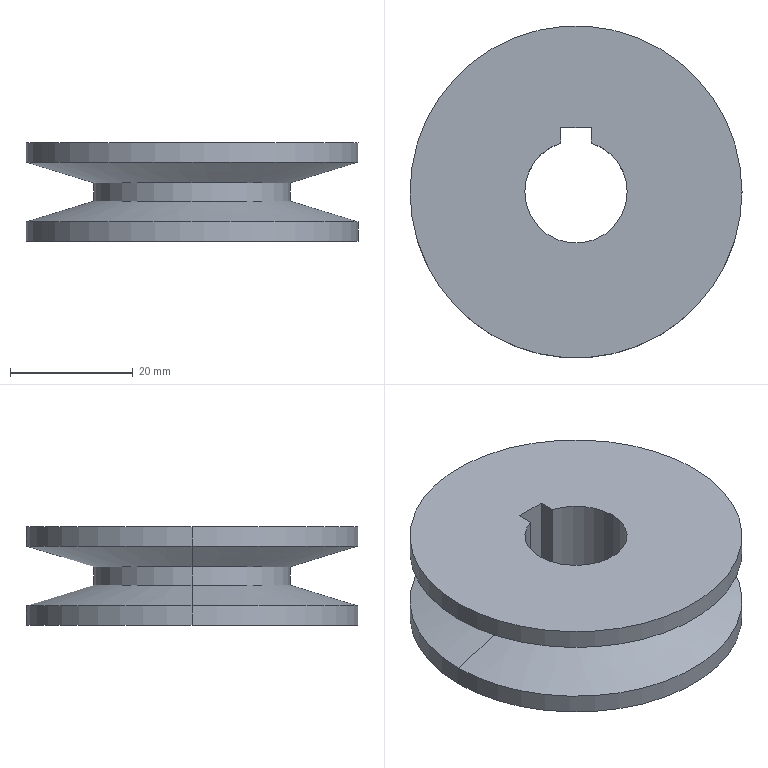Part | SolidWorks | features ICE 2, BaseBody 1 | 1 solid | 18 faces | box 54 x 54 x 16 mm | volume 23103 mm3 | cylinder 9 | plane 5 | cone 4 | commonest cylinder face diameters 54 x4 16.64 x3 32 x2
STEP:
#1=CARTESIAN_POINT('',(-8.32,0.,0.));
#2=VERTEX_POINT('',#1);
#3=CARTESIAN_POINT('',(8.32,0.,0.));
#4=VERTEX_POINT('',#3);
#5=CARTESIAN_POINT('',(0.,0.,0.));
#6=DIRECTION('',(0.,0.,1.));
#7=DIRECTION('',(1.,0.,0.));
#8=AXIS2_PLACEMENT_3D('',#5,#6,#7);
#9=CIRCLE('',#8,8.32);
#10=EDGE_CURVE('',#2,#4,#9,.T.);
#11=ORIENTED_EDGE('',*,*,#10,.F.);
#12=CARTESIAN_POINT('',(-8.32,0.,16.));
#13=VERTEX_POINT('',#12);
#14=CARTESIAN_POINT('',(-8.32,0.,0.));
#15=DIRECTION('',(0.,0.,1.));
#16=VECTOR('',#15,1000.);
#17=LINE('',#14,#16);
#18=EDGE_CURVE('',#2,#13,#17,.T.);
#19=ORIENTED_EDGE('',*,*,#18,.T.);
#20=CARTESIAN_POINT('',(8.32,0.,16.));
#21=VERTEX_POINT('',#20);
#22=CARTESIAN_POINT('',(0.,0.,16.));
#23=DIRECTION('',(0.,0.,1.));
#24=DIRECTION('',(1.,0.,0.));
#25=AXIS2_PLACEMENT_3D('',#22,#23,#24);
#26=CIRCLE('',#25,8.32);
#27=EDGE_CURVE('',#13,#21,#26,.T.);
#28=ORIENTED_EDGE('',*,*,#27,.T.);
#29=CARTESIAN_POINT('',(8.32,0.,0.));
#30=DIRECTION('',(0.,0.,1.));
#31=VECTOR('',#30,1000.);
#32=LINE('',#29,#31);
#33=EDGE_CURVE('',#4,#21,#32,.T.);
#34=ORIENTED_EDGE('',*,*,#33,.F.);
#35=EDGE_LOOP('',(#11,#19,#28,#34));
#36=FACE_OUTER_BOUND('',#35,.T.);
#37=CARTESIAN_POINT('',(0.,0.,0.));
#38=DIRECTION('',(0.,0.,1.));
#39=DIRECTION('',(1.,0.,0.));
#40=AXIS2_PLACEMENT_3D('',#37,#38,#39);
#41=CYLINDRICAL_SURFACE('',#40,8.32);
#42=ADVANCED_FACE('',(#36),#41,.F.);
#43=CARTESIAN_POINT('',(2.5,7.936,0.));
#44=VERTEX_POINT('',#43);
#45=CARTESIAN_POINT('',(0.,0.,0.));
#46=DIRECTION('',(0.,0.,1.));
#47=DIRECTION('',(1.,0.,0.));
#48=AXIS2_PLACEMENT_3D('',#45,#46,#47);
#49=CIRCLE('',#48,8.32);
#50=EDGE_CURVE('',#4,#44,#49,.T.);
#51=ORIENTED_EDGE('',*,*,#50,.F.);
#52=ORIENTED_EDGE('',*,*,#33,.T.);
#53=CARTESIAN_POINT('',(2.5,7.936,16.));
#54=VERTEX_POINT('',#53);
#55=CARTESIAN_POINT('',(0.,0.,16.));
#56=DIRECTION('',(0.,0.,1.));
#57=DIRECTION('',(1.,0.,0.));
#58=AXIS2_PLACEMENT_3D('',#55,#56,#57);
#59=CIRCLE('',#58,8.32);
#60=EDGE_CURVE('',#21,#54,#59,.T.);
#61=ORIENTED_EDGE('',*,*,#60,.T.);
#62=CARTESIAN_POINT('',(2.5,7.936,0.));
#63=DIRECTION('',(0.,0.,-1.));
#64=VECTOR('',#63,1000.);
#65=LINE('',#62,#64);
#66=EDGE_CURVE('',#54,#44,#65,.T.);
#67=ORIENTED_EDGE('',*,*,#66,.T.);
#68=EDGE_LOOP('',(#51,#52,#61,#67));
#69=FACE_OUTER_BOUND('',#68,.T.);
#70=CARTESIAN_POINT('',(0.,0.,0.));
#71=DIRECTION('',(0.,0.,1.));
#72=DIRECTION('',(1.,0.,0.));
#73=AXIS2_PLACEMENT_3D('',#70,#71,#72);
#74=CYLINDRICAL_SURFACE('',#73,8.32);
#75=ADVANCED_FACE('',(#69),#74,.F.);
#76=CARTESIAN_POINT('',(27.,0.,16.));
#77=VERTEX_POINT('',#76);
#78=CARTESIAN_POINT('',(-27.,0.,16.));
#79=VERTEX_POINT('',#78);
#80=CARTESIAN_POINT('',(0.,0.,16.));
#81=DIRECTION('',(0.,0.,1.));
#82=DIRECTION('',(-1.,0.,0.));
#83=AXIS2_PLACEMENT_3D('',#80,#81,#82);
#84=CIRCLE('',#83,27.);
#85=EDGE_CURVE('',#77,#79,#84,.T.);
#86=ORIENTED_EDGE('',*,*,#85,.F.);
#87=CARTESIAN_POINT('',(27.,0.,12.861));
#88=VERTEX_POINT('',#87);
#89=CARTESIAN_POINT('',(27.,0.,8.));
#90=DIRECTION('',(0.,0.,-1.));
#91=VECTOR('',#90,1000.);
#92=LINE('',#89,#91);
#93=EDGE_CURVE('',#77,#88,#92,.T.);
#94=ORIENTED_EDGE('',*,*,#93,.T.);
#95=CARTESIAN_POINT('',(-27.,0.,12.861));
#96=VERTEX_POINT('',#95);
#97=CARTESIAN_POINT('',(0.,0.,12.861));
#98=DIRECTION('',(0.,0.,1.));
#99=DIRECTION('',(-1.,0.,0.));
#100=AXIS2_PLACEMENT_3D('',#97,#98,#99);
#101=CIRCLE('',#100,27.);
#102=EDGE_CURVE('',#88,#96,#101,.T.);
#103=ORIENTED_EDGE('',*,*,#102,.T.);
#104=CARTESIAN_POINT('',(-27.,0.,8.));
#105=DIRECTION('',(0.,0.,-1.));
#106=VECTOR('',#105,1000.);
#107=LINE('',#104,#106);
#108=EDGE_CURVE('',#79,#96,#107,.T.);
#109=ORIENTED_EDGE('',*,*,#108,.F.);
#110=EDGE_LOOP('',(#86,#94,#103,#109));
#111=FACE_OUTER_BOUND('',#110,.T.);
#112=CARTESIAN_POINT('',(0.,0.,8.));
#113=DIRECTION('',(0.,0.,-1.));
#114=DIRECTION('',(-1.,0.,0.));
#115=AXIS2_PLACEMENT_3D('',#112,#113,#114);
#116=CYLINDRICAL_SURFACE('',#115,27.);
#117=ADVANCED_FACE('',(#111),#116,.T.);
#118=CARTESIAN_POINT('',(16.,0.,9.498));
#119=VERTEX_POINT('',#118);
#120=CARTESIAN_POINT('',(-16.,0.,9.498));
#121=VERTEX_POINT('',#120);
#122=CARTESIAN_POINT('',(0.,0.,9.498));
#123=DIRECTION('',(0.,0.,1.));
#124=DIRECTION('',(0.,1.,0.));
#125=AXIS2_PLACEMENT_3D('',#122,#123,#124);
#126=CIRCLE('',#125,16.);
#127=EDGE_CURVE('',#119,#121,#126,.T.);
#128=ORIENTED_EDGE('',*,*,#127,.T.);
#129=CARTESIAN_POINT('',(-27.,0.,12.861));
#130=DIRECTION('',(-0.9563,0.,0.2924));
#131=VECTOR('',#130,1000.);
#132=LINE('',#129,#131);
#133=EDGE_CURVE('',#121,#96,#132,.T.);
#134=ORIENTED_EDGE('',*,*,#133,.T.);
#135=ORIENTED_EDGE('',*,*,#102,.F.);
#136=CARTESIAN_POINT('',(27.,0.,12.861));
#137=DIRECTION('',(0.9563,0.,0.2924));
#138=VECTOR('',#137,1000.);
#139=LINE('',#136,#138);
#140=EDGE_CURVE('',#119,#88,#139,.T.);
#141=ORIENTED_EDGE('',*,*,#140,.F.);
#142=EDGE_LOOP('',(#128,#134,#135,#141));
#143=FACE_OUTER_BOUND('',#142,.T.);
#144=CARTESIAN_POINT('',(0.,0.,12.861));
#145=DIRECTION('',(0.,0.,1.));
#146=DIRECTION('',(1.,0.,0.));
#147=AXIS2_PLACEMENT_3D('',#144,#145,#146);
#148=CONICAL_SURFACE('',#147,27.,1.274);
#149=ADVANCED_FACE('',(#143),#148,.T.);
#150=CARTESIAN_POINT('',(16.,0.,6.502));
#151=VERTEX_POINT('',#150);
#152=CARTESIAN_POINT('',(-16.,0.,6.502));
#153=VERTEX_POINT('',#152);
#154=CARTESIAN_POINT('',(0.,0.,6.502));
#155=DIRECTION('',(0.,0.,1.));
#156=DIRECTION('',(1.,0.,0.));
#157=AXIS2_PLACEMENT_3D('',#154,#155,#156);
#158=CIRCLE('',#157,16.);
#159=EDGE_CURVE('',#151,#153,#158,.T.);
#160=ORIENTED_EDGE('',*,*,#159,.T.);
#161=CARTESIAN_POINT('',(-16.,0.,8.));
#162=DIRECTION('',(0.,0.,1.));
#163=VECTOR('',#162,1000.);
#164=LINE('',#161,#163);
#165=EDGE_CURVE('',#153,#121,#164,.T.);
#166=ORIENTED_EDGE('',*,*,#165,.T.);
#167=ORIENTED_EDGE('',*,*,#127,.F.);
#168=CARTESIAN_POINT('',(16.,0.,8.));
#169=DIRECTION('',(0.,0.,1.));
#170=VECTOR('',#169,1000.);
#171=LINE('',#168,#170);
#172=EDGE_CURVE('',#151,#119,#171,.T.);
#173=ORIENTED_EDGE('',*,*,#172,.F.);
#174=EDGE_LOOP('',(#160,#166,#167,#173));
#175=FACE_OUTER_BOUND('',#174,.T.);
#176=CARTESIAN_POINT('',(0.,0.,8.));
#177=DIRECTION('',(0.,0.,1.));
#178=DIRECTION('',(1.,0.,0.));
#179=AXIS2_PLACEMENT_3D('',#176,#177,#178);
#180=CYLINDRICAL_SURFACE('',#179,16.);
#181=ADVANCED_FACE('',(#175),#180,.T.);
#182=ORIENTED_EDGE('',*,*,#159,.F.);
#183=CARTESIAN_POINT('',(27.,0.,3.139));
#184=VERTEX_POINT('',#183);
#185=CARTESIAN_POINT('',(27.,0.,3.139));
#186=DIRECTION('',(0.9563,0.,-0.2924));
#187=VECTOR('',#186,1000.);
#188=LINE('',#185,#187);
#189=EDGE_CURVE('',#151,#184,#188,.T.);
#190=ORIENTED_EDGE('',*,*,#189,.T.);
#191=CARTESIAN_POINT('',(-27.,0.,3.139));
#192=VERTEX_POINT('',#191);
#193=CARTESIAN_POINT('',(0.,0.,3.139));
#194=DIRECTION('',(0.,0.,1.));
#195=DIRECTION('',(0.,1.,0.));
#196=AXIS2_PLACEMENT_3D('',#193,#194,#195);
#197=CIRCLE('',#196,27.);
#198=EDGE_CURVE('',#184,#192,#197,.T.);
#199=ORIENTED_EDGE('',*,*,#198,.T.);
#200=CARTESIAN_POINT('',(-27.,0.,3.139));
#201=DIRECTION('',(-0.9563,0.,-0.2924));
#202=VECTOR('',#201,1000.);
#203=LINE('',#200,#202);
#204=EDGE_CURVE('',#153,#192,#203,.T.);
#205=ORIENTED_EDGE('',*,*,#204,.F.);
#206=EDGE_LOOP('',(#182,#190,#199,#205));
#207=FACE_OUTER_BOUND('',#206,.T.);
#208=CARTESIAN_POINT('',(0.,0.,3.139));
#209=DIRECTION('',(0.,0.,-1.));
#210=DIRECTION('',(-1.,0.,0.));
#211=AXIS2_PLACEMENT_3D('',#208,#209,#210);
#212=CONICAL_SURFACE('',#211,27.,1.274);
#213=ADVANCED_FACE('',(#207),#212,.T.);
#214=ORIENTED_EDGE('',*,*,#198,.F.);
#215=CARTESIAN_POINT('',(27.,0.,0.));
#216=VERTEX_POINT('',#215);
#217=CARTESIAN_POINT('',(27.,0.,8.));
#218=DIRECTION('',(0.,0.,-1.));
#219=VECTOR('',#218,1000.);
#220=LINE('',#217,#219);
#221=EDGE_CURVE('',#184,#216,#220,.T.);
#222=ORIENTED_EDGE('',*,*,#221,.T.);
#223=CARTESIAN_POINT('',(-27.,0.,0.));
#224=VERTEX_POINT('',#223);
#225=CARTESIAN_POINT('',(0.,0.,0.));
#226=DIRECTION('',(0.,0.,1.));
#227=DIRECTION('',(-1.,0.,0.));
#228=AXIS2_PLACEMENT_3D('',#225,#226,#227);
#229=CIRCLE('',#228,27.);
#230=EDGE_CURVE('',#216,#224,#229,.T.);
#231=ORIENTED_EDGE('',*,*,#230,.T.);
#232=CARTESIAN_POINT('',(-27.,0.,8.));
#233=DIRECTION('',(0.,0.,-1.));
#234=VECTOR('',#233,1000.);
#235=LINE('',#232,#234);
#236=EDGE_CURVE('',#192,#224,#235,.T.);
#237=ORIENTED_EDGE('',*,*,#236,.F.);
#238=EDGE_LOOP('',(#214,#222,#231,#237));
#239=FACE_OUTER_BOUND('',#238,.T.);
#240=CARTESIAN_POINT('',(0.,0.,8.));
#241=DIRECTION('',(0.,0.,-1.));
#242=DIRECTION('',(-1.,0.,0.));
#243=AXIS2_PLACEMENT_3D('',#240,#241,#242);
#244=CYLINDRICAL_SURFACE('',#243,27.);
#245=ADVANCED_FACE('',(#239),#244,.T.);
#246=CARTESIAN_POINT('',(-2.5,10.5,16.));
#247=VERTEX_POINT('',#246);
#248=CARTESIAN_POINT('',(-2.5,7.936,16.));
#249=VERTEX_POINT('',#248);
#250=CARTESIAN_POINT('',(-2.5,10.5,16.));
#251=DIRECTION('',(0.,-1.,0.));
#252=VECTOR('',#251,1000.);
#253=LINE('',#250,#252);
#254=EDGE_CURVE('',#247,#249,#253,.T.);
#255=ORIENTED_EDGE('',*,*,#254,.F.);
#256=CARTESIAN_POINT('',(2.5,10.5,16.));
#257=VERTEX_POINT('',#256);
#258=CARTESIAN_POINT('',(-2.5,10.5,16.));
#259=DIRECTION('',(-1.,0.,0.));
#260=VECTOR('',#259,1000.);
#261=LINE('',#258,#260);
#262=EDGE_CURVE('',#257,#247,#261,.T.);
#263=ORIENTED_EDGE('',*,*,#262,.F.);
#264=CARTESIAN_POINT('',(2.5,10.5,16.));
#265=DIRECTION('',(0.,1.,0.));
#266=VECTOR('',#265,1000.);
#267=LINE('',#264,#266);
#268=EDGE_CURVE('',#54,#257,#267,.T.);
#269=ORIENTED_EDGE('',*,*,#268,.F.);
#270=ORIENTED_EDGE('',*,*,#60,.F.);
#271=ORIENTED_EDGE('',*,*,#27,.F.);
#272=CARTESIAN_POINT('',(0.,0.,16.));
#273=DIRECTION('',(0.,0.,1.));
#274=DIRECTION('',(1.,0.,0.));
#275=AXIS2_PLACEMENT_3D('',#272,#273,#274);
#276=CIRCLE('',#275,8.32);
#277=EDGE_CURVE('',#249,#13,#276,.T.);
#278=ORIENTED_EDGE('',*,*,#277,.F.);
#279=EDGE_LOOP('',(#255,#263,#269,#270,#271,#278));
#280=FACE_BOUND('',#279,.T.);
#281=CARTESIAN_POINT('',(0.,0.,16.));
#282=DIRECTION('',(0.,0.,1.));
#283=DIRECTION('',(-1.,0.,0.));
#284=AXIS2_PLACEMENT_3D('',#281,#282,#283);
#285=CIRCLE('',#284,27.);
#286=EDGE_CURVE('',#79,#77,#285,.T.);
#287=ORIENTED_EDGE('',*,*,#286,.T.);
#288=ORIENTED_EDGE('',*,*,#85,.T.);
#289=EDGE_LOOP('',(#287,#288));
#290=FACE_OUTER_BOUND('',#289,.T.);
#291=CARTESIAN_POINT('',(0.,13.5,16.));
#292=DIRECTION('',(0.,0.,1.));
#293=DIRECTION('',(1.,0.,0.));
#294=AXIS2_PLACEMENT_3D('',#291,#292,#293);
#295=PLANE('',#294);
#296=ADVANCED_FACE('',(#280,#290),#295,.T.);
#297=ORIENTED_EDGE('',*,*,#93,.F.);
#298=ORIENTED_EDGE('',*,*,#286,.F.);
#299=ORIENTED_EDGE('',*,*,#108,.T.);
#300=CARTESIAN_POINT('',(0.,0.,12.861));
#301=DIRECTION('',(0.,0.,1.));
#302=DIRECTION('',(-1.,0.,0.));
#303=AXIS2_PLACEMENT_3D('',#300,#301,#302);
#304=CIRCLE('',#303,27.);
#305=EDGE_CURVE('',#96,#88,#304,.T.);
#306=ORIENTED_EDGE('',*,*,#305,.T.);
#307=EDGE_LOOP('',(#297,#298,#299,#306));
#308=FACE_OUTER_BOUND('',#307,.T.);
#309=CARTESIAN_POINT('',(0.,0.,8.));
#310=DIRECTION('',(0.,0.,-1.));
#311=DIRECTION('',(-1.,0.,0.));
#312=AXIS2_PLACEMENT_3D('',#309,#310,#311);
#313=CYLINDRICAL_SURFACE('',#312,27.);
#314=ADVANCED_FACE('',(#308),#313,.T.);
#315=ORIENTED_EDGE('',*,*,#133,.F.);
#316=CARTESIAN_POINT('',(0.,0.,9.498));
#317=DIRECTION('',(0.,0.,1.));
#318=DIRECTION('',(0.,1.,0.));
#319=AXIS2_PLACEMENT_3D('',#316,#317,#318);
#320=CIRCLE('',#319,16.);
#321=EDGE_CURVE('',#121,#119,#320,.T.);
#322=ORIENTED_EDGE('',*,*,#321,.T.);
#323=ORIENTED_EDGE('',*,*,#140,.T.);
#324=ORIENTED_EDGE('',*,*,#305,.F.);
#325=EDGE_LOOP('',(#315,#322,#323,#324));
#326=FACE_OUTER_BOUND('',#325,.T.);
#327=CARTESIAN_POINT('',(0.,0.,12.861));
#328=DIRECTION('',(0.,0.,1.));
#329=DIRECTION('',(1.,0.,0.));
#330=AXIS2_PLACEMENT_3D('',#327,#328,#329);
#331=CONICAL_SURFACE('',#330,27.,1.274);
#332=ADVANCED_FACE('',(#326),#331,.T.);
#333=ORIENTED_EDGE('',*,*,#165,.F.);
#334=CARTESIAN_POINT('',(0.,0.,6.502));
#335=DIRECTION('',(0.,0.,1.));
#336=DIRECTION('',(1.,0.,0.));
#337=AXIS2_PLACEMENT_3D('',#334,#335,#336);
#338=CIRCLE('',#337,16.);
#339=EDGE_CURVE('',#153,#151,#338,.T.);
#340=ORIENTED_EDGE('',*,*,#339,.T.);
#341=ORIENTED_EDGE('',*,*,#172,.T.);
#342=ORIENTED_EDGE('',*,*,#321,.F.);
#343=EDGE_LOOP('',(#333,#340,#341,#342));
#344=FACE_OUTER_BOUND('',#343,.T.);
#345=CARTESIAN_POINT('',(0.,0.,8.));
#346=DIRECTION('',(0.,0.,1.));
#347=DIRECTION('',(1.,0.,0.));
#348=AXIS2_PLACEMENT_3D('',#345,#346,#347);
#349=CYLINDRICAL_SURFACE('',#348,16.);
#350=ADVANCED_FACE('',(#344),#349,.T.);
#351=ORIENTED_EDGE('',*,*,#189,.F.);
#352=ORIENTED_EDGE('',*,*,#339,.F.);
#353=ORIENTED_EDGE('',*,*,#204,.T.);
#354=CARTESIAN_POINT('',(0.,0.,3.139));
#355=DIRECTION('',(0.,0.,1.));
#356=DIRECTION('',(0.,1.,0.));
#357=AXIS2_PLACEMENT_3D('',#354,#355,#356);
#358=CIRCLE('',#357,27.);
#359=EDGE_CURVE('',#192,#184,#358,.T.);
#360=ORIENTED_EDGE('',*,*,#359,.T.);
#361=EDGE_LOOP('',(#351,#352,#353,#360));
#362=FACE_OUTER_BOUND('',#361,.T.);
#363=CARTESIAN_POINT('',(0.,0.,3.139));
#364=DIRECTION('',(0.,0.,-1.));
#365=DIRECTION('',(-1.,0.,0.));
#366=AXIS2_PLACEMENT_3D('',#363,#364,#365);
#367=CONICAL_SURFACE('',#366,27.,1.274);
#368=ADVANCED_FACE('',(#362),#367,.T.);
#369=ORIENTED_EDGE('',*,*,#221,.F.);
#370=ORIENTED_EDGE('',*,*,#359,.F.);
#371=ORIENTED_EDGE('',*,*,#236,.T.);
#372=CARTESIAN_POINT('',(0.,0.,0.));
#373=DIRECTION('',(0.,0.,1.));
#374=DIRECTION('',(-1.,0.,0.));
#375=AXIS2_PLACEMENT_3D('',#372,#373,#374);
#376=CIRCLE('',#375,27.);
#377=EDGE_CURVE('',#224,#216,#376,.T.);
#378=ORIENTED_EDGE('',*,*,#377,.T.);
#379=EDGE_LOOP('',(#369,#370,#371,#378));
#380=FACE_OUTER_BOUND('',#379,.T.);
#381=CARTESIAN_POINT('',(0.,0.,8.));
#382=DIRECTION('',(0.,0.,-1.));
#383=DIRECTION('',(-1.,0.,0.));
#384=AXIS2_PLACEMENT_3D('',#381,#382,#383);
#385=CYLINDRICAL_SURFACE('',#384,27.);
#386=ADVANCED_FACE('',(#380),#385,.T.);
#387=CARTESIAN_POINT('',(-2.5,10.5,0.));
#388=VERTEX_POINT('',#387);
#389=CARTESIAN_POINT('',(-2.5,7.936,0.));
#390=VERTEX_POINT('',#389);
#391=CARTESIAN_POINT('',(-2.5,10.5,0.));
#392=DIRECTION('',(0.,-1.,0.));
#393=VECTOR('',#392,1000.);
#394=LINE('',#391,#393);
#395=EDGE_CURVE('',#388,#390,#394,.T.);
#396=ORIENTED_EDGE('',*,*,#395,.T.);
#397=CARTESIAN_POINT('',(0.,0.,0.));
#398=DIRECTION('',(0.,0.,1.));
#399=DIRECTION('',(1.,0.,0.));
#400=AXIS2_PLACEMENT_3D('',#397,#398,#399);
#401=CIRCLE('',#400,8.32);
#402=EDGE_CURVE('',#390,#2,#401,.T.);
#403=ORIENTED_EDGE('',*,*,#402,.T.);
#404=ORIENTED_EDGE('',*,*,#10,.T.);
#405=ORIENTED_EDGE('',*,*,#50,.T.);
#406=CARTESIAN_POINT('',(2.5,10.5,0.));
#407=VERTEX_POINT('',#406);
#408=CARTESIAN_POINT('',(2.5,10.5,0.));
#409=DIRECTION('',(0.,1.,0.));
#410=VECTOR('',#409,1000.);
#411=LINE('',#408,#410);
#412=EDGE_CURVE('',#44,#407,#411,.T.);
#413=ORIENTED_EDGE('',*,*,#412,.T.);
#414=CARTESIAN_POINT('',(-2.5,10.5,0.));
#415=DIRECTION('',(-1.,0.,0.));
#416=VECTOR('',#415,1000.);
#417=LINE('',#414,#416);
#418=EDGE_CURVE('',#407,#388,#417,.T.);
#419=ORIENTED_EDGE('',*,*,#418,.T.);
#420=EDGE_LOOP('',(#396,#403,#404,#405,#413,#419));
#421=FACE_BOUND('',#420,.T.);
#422=ORIENTED_EDGE('',*,*,#377,.F.);
#423=ORIENTED_EDGE('',*,*,#230,.F.);
#424=EDGE_LOOP('',(#422,#423));
#425=FACE_OUTER_BOUND('',#424,.T.);
#426=CARTESIAN_POINT('',(0.,13.5,0.));
#427=DIRECTION('',(0.,0.,-1.));
#428=DIRECTION('',(-1.,0.,0.));
#429=AXIS2_PLACEMENT_3D('',#426,#427,#428);
#430=PLANE('',#429);
#431=ADVANCED_FACE('',(#421,#425),#430,.T.);
#432=ORIENTED_EDGE('',*,*,#18,.F.);
#433=ORIENTED_EDGE('',*,*,#402,.F.);
#434=CARTESIAN_POINT('',(-2.5,7.936,0.));
#435=DIRECTION('',(0.,0.,1.));
#436=VECTOR('',#435,1000.);
#437=LINE('',#434,#436);
#438=EDGE_CURVE('',#390,#249,#437,.T.);
#439=ORIENTED_EDGE('',*,*,#438,.T.);
#440=ORIENTED_EDGE('',*,*,#277,.T.);
#441=EDGE_LOOP('',(#432,#433,#439,#440));
#442=FACE_OUTER_BOUND('',#441,.T.);
#443=CARTESIAN_POINT('',(0.,0.,0.));
#444=DIRECTION('',(0.,0.,1.));
#445=DIRECTION('',(1.,0.,0.));
#446=AXIS2_PLACEMENT_3D('',#443,#444,#445);
#447=CYLINDRICAL_SURFACE('',#446,8.32);
#448=ADVANCED_FACE('',(#442),#447,.F.);
#449=ORIENTED_EDGE('',*,*,#395,.F.);
#450=CARTESIAN_POINT('',(-2.5,10.5,0.));
#451=DIRECTION('',(0.,0.,1.));
#452=VECTOR('',#451,1000.);
#453=LINE('',#450,#452);
#454=EDGE_CURVE('',#388,#247,#453,.T.);
#455=ORIENTED_EDGE('',*,*,#454,.T.);
#456=ORIENTED_EDGE('',*,*,#254,.T.);
#457=ORIENTED_EDGE('',*,*,#438,.F.);
#458=EDGE_LOOP('',(#449,#455,#456,#457));
#459=FACE_OUTER_BOUND('',#458,.T.);
#460=CARTESIAN_POINT('',(-2.5,10.5,0.));
#461=DIRECTION('',(-1.,0.,0.));
#462=DIRECTION('',(0.,-1.,0.));
#463=AXIS2_PLACEMENT_3D('',#460,#461,#462);
#464=PLANE('',#463);
#465=ADVANCED_FACE('',(#459),#464,.F.);
#466=ORIENTED_EDGE('',*,*,#268,.T.);
#467=CARTESIAN_POINT('',(2.5,10.5,0.));
#468=DIRECTION('',(0.,0.,1.));
#469=VECTOR('',#468,1000.);
#470=LINE('',#467,#469);
#471=EDGE_CURVE('',#407,#257,#470,.T.);
#472=ORIENTED_EDGE('',*,*,#471,.F.);
#473=ORIENTED_EDGE('',*,*,#412,.F.);
#474=ORIENTED_EDGE('',*,*,#66,.F.);
#475=EDGE_LOOP('',(#466,#472,#473,#474));
#476=FACE_OUTER_BOUND('',#475,.T.);
#477=CARTESIAN_POINT('',(2.5,10.5,0.));
#478=DIRECTION('',(1.,0.,0.));
#479=DIRECTION('',(0.,1.,0.));
#480=AXIS2_PLACEMENT_3D('',#477,#478,#479);
#481=PLANE('',#480);
#482=ADVANCED_FACE('',(#476),#481,.F.);
#483=ORIENTED_EDGE('',*,*,#262,.T.);
#484=ORIENTED_EDGE('',*,*,#454,.F.);
#485=ORIENTED_EDGE('',*,*,#418,.F.);
#486=ORIENTED_EDGE('',*,*,#471,.T.);
#487=EDGE_LOOP('',(#483,#484,#485,#486));
#488=FACE_OUTER_BOUND('',#487,.T.);
#489=CARTESIAN_POINT('',(-2.5,10.5,0.));
#490=DIRECTION('',(0.,1.,0.));
#491=DIRECTION('',(0.,0.,1.));
#492=AXIS2_PLACEMENT_3D('',#489,#490,#491);
#493=PLANE('',#492);
#494=ADVANCED_FACE('',(#488),#493,.F.);
#495=CLOSED_SHELL('',(#42,#75,#117,#149,#181,#213,#245,#296,#314,#332,#350,#368,#386,#431,#448,#465,#482,#494));
#496=MANIFOLD_SOLID_BREP('',#495);
#497=CARTESIAN_POINT('',(0.,0.,0.));
#498=DIRECTION('',(0.,0.,1.));
#499=DIRECTION('',(1.,0.,0.));
#500=AXIS2_PLACEMENT_3D('',#497,#498,#499);
#501=(LENGTH_UNIT()NAMED_UNIT(*)SI_UNIT(.MILLI.,.METRE.));
#502=UNCERTAINTY_MEASURE_WITH_UNIT(LENGTH_MEASURE(0.00001),#501,'','');
#503=(NAMED_UNIT(*)PLANE_ANGLE_UNIT()SI_UNIT($,.RADIAN.));
#504=(NAMED_UNIT(*)SI_UNIT($,.STERADIAN.)SOLID_ANGLE_UNIT());
#505=(GEOMETRIC_REPRESENTATION_CONTEXT(3)GLOBAL_UNCERTAINTY_ASSIGNED_CONTEXT((#502))GLOBAL_UNIT_ASSIGNED_CONTEXT((#501,#503,#504))REPRESENTATION_CONTEXT('',''));
#506=ADVANCED_BREP_SHAPE_REPRESENTATION('',(#496,#500),#505);